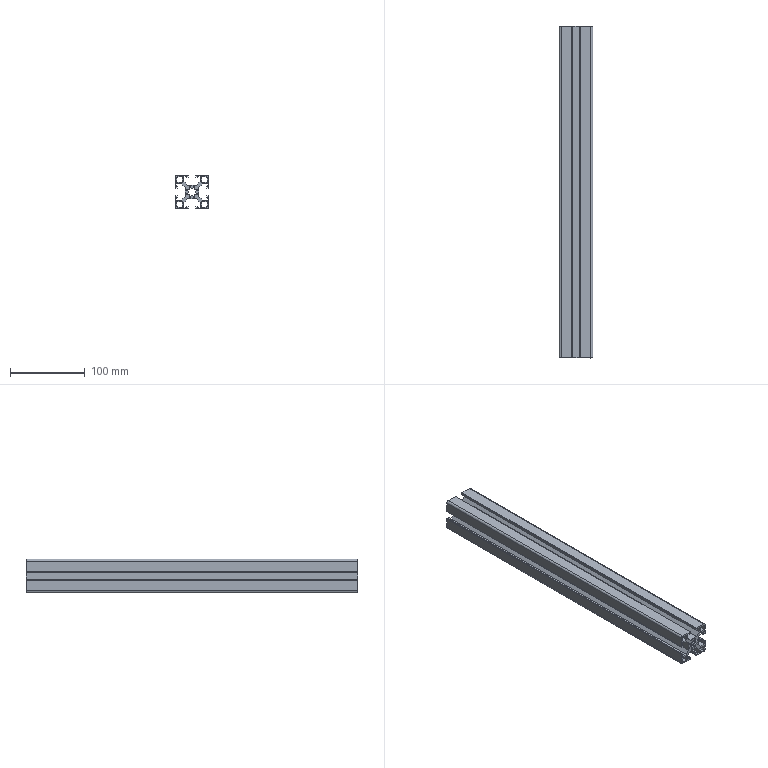Part | STEP file | 1 solid | 135 faces | box 45 x 445 x 45 mm | volume 308069 mm3 | plane 118 | cylinder 17 | commonest cylinder face diameters 10 x9 3 x4 5 x4